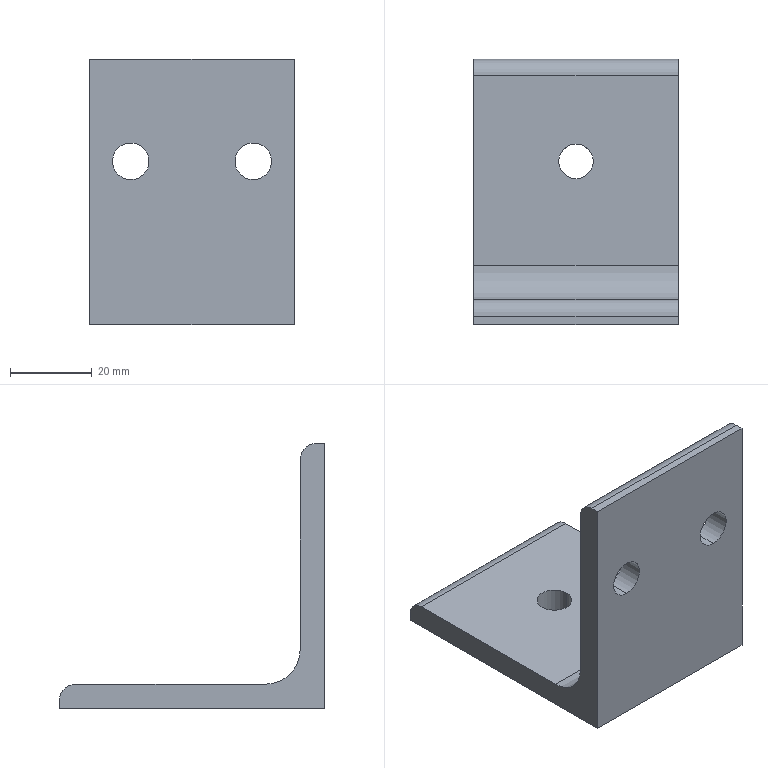Part | STEP file | 0245_204_Blacket | 1 solid | 17 faces | box 50 x 65 x 65 mm | volume 36528 mm3 | cylinder 9 | plane 8 | commonest cylinder face diameters 9 x4 8 x2 8.5 x2 17 x1
STEP:
#1=CARTESIAN_POINT('',(0.,0.,0.));
#2=DIRECTION('',(0.,0.,1.));
#3=DIRECTION('',(1.,0.,0.));
#4=AXIS2_PLACEMENT_3D('',#1,#2,#3);
#5=CARTESIAN_POINT('',(4.25,40.,-65.));
#6=VERTEX_POINT('',#5);
#7=CARTESIAN_POINT('',(4.25,40.,-59.));
#8=VERTEX_POINT('',#7);
#9=CARTESIAN_POINT('',(4.25,40.,-59.));
#10=DIRECTION('',(0.,0.,1.));
#11=VECTOR('',#10,1.);
#12=LINE('',#9,#11);
#13=CARTESIAN_POINT('',(0.,40.,-59.));
#14=DIRECTION('',(0.,0.,1.));
#15=DIRECTION('',(1.,0.,0.));
#16=AXIS2_PLACEMENT_3D('',#13,#14,#15);
#17=CYLINDRICAL_SURFACE('',#16,4.25);
#18=CARTESIAN_POINT('',(6.283,0.));
#19=DIRECTION('',(0.,1.));
#20=VECTOR('',#19,1.);
#21=LINE('',#18,#20);
#22=(GEOMETRIC_REPRESENTATION_CONTEXT(2)PARAMETRIC_REPRESENTATION_CONTEXT()REPRESENTATION_CONTEXT('',''));
#23=DEFINITIONAL_REPRESENTATION('',(#21),#22);
#24=PCURVE('',#17,#23);
#25=CARTESIAN_POINT('',(0.,40.,-59.));
#26=DIRECTION('',(0.,0.,1.));
#27=DIRECTION('',(1.,0.,0.));
#28=AXIS2_PLACEMENT_3D('',#25,#26,#27);
#29=CYLINDRICAL_SURFACE('',#28,4.25);
#30=CARTESIAN_POINT('',(0.,0.));
#31=DIRECTION('',(0.,1.));
#32=VECTOR('',#31,1.);
#33=LINE('',#30,#32);
#34=(GEOMETRIC_REPRESENTATION_CONTEXT(2)PARAMETRIC_REPRESENTATION_CONTEXT()REPRESENTATION_CONTEXT('',''));
#35=DEFINITIONAL_REPRESENTATION('',(#33),#34);
#36=PCURVE('',#29,#35);
#37=SURFACE_CURVE('',#12,(#24,#36),.PCURVE_S1.);
#38=EDGE_CURVE('',#6,#8,#37,.T.);
#39=ORIENTED_EDGE('',*,*,#38,.T.);
#40=CARTESIAN_POINT('',(-4.25,40.,-59.));
#41=VERTEX_POINT('',#40);
#42=CARTESIAN_POINT('',(0.,40.,-59.));
#43=DIRECTION('',(0.,0.,1.));
#44=DIRECTION('',(1.,0.,0.));
#45=AXIS2_PLACEMENT_3D('',#42,#43,#44);
#46=CIRCLE('',#45,4.25);
#47=CARTESIAN_POINT('',(0.,0.));
#48=DIRECTION('',(1.,0.));
#49=VECTOR('',#48,1.);
#50=LINE('',#47,#49);
#51=(GEOMETRIC_REPRESENTATION_CONTEXT(2)PARAMETRIC_REPRESENTATION_CONTEXT()REPRESENTATION_CONTEXT('',''));
#52=DEFINITIONAL_REPRESENTATION('',(#50),#51);
#53=PCURVE('',#17,#52);
#54=CARTESIAN_POINT('',(25.,65.,-59.));
#55=DIRECTION('',(0.,0.,-1.));
#56=DIRECTION('',(0.,1.,0.));
#57=AXIS2_PLACEMENT_3D('',#54,#55,#56);
#58=PLANE('',#57);
#59=CARTESIAN_POINT('',(-25.,-20.75));
#60=CARTESIAN_POINT('',(-17.639,-20.75));
#61=CARTESIAN_POINT('',(-21.319,-27.125));
#62=CARTESIAN_POINT('',(-25.,-33.5));
#63=CARTESIAN_POINT('',(-28.681,-27.125));
#64=CARTESIAN_POINT('',(-32.361,-20.75));
#65=CARTESIAN_POINT('',(-25.,-20.75));
#66=(BOUNDED_CURVE()B_SPLINE_CURVE(2,(#59,#60,#61,#62,#63,#64,#65),.UNSPECIFIED.,.T.,.F.)B_SPLINE_CURVE_WITH_KNOTS((1,2,2,2,2,1),(-2.094,0.,2.094,4.189,6.283,8.378),.UNSPECIFIED.)CURVE()GEOMETRIC_REPRESENTATION_ITEM()RATIONAL_B_SPLINE_CURVE((1.,0.5,1.,0.5,1.,0.5,1.))REPRESENTATION_ITEM(''));
#67=(GEOMETRIC_REPRESENTATION_CONTEXT(2)PARAMETRIC_REPRESENTATION_CONTEXT()REPRESENTATION_CONTEXT('',''));
#68=DEFINITIONAL_REPRESENTATION('',(#66),#67);
#69=PCURVE('',#58,#68);
#70=SURFACE_CURVE('',#46,(#53,#69),.PCURVE_S1.);
#71=EDGE_CURVE('',#41,#8,#70,.T.);
#72=ORIENTED_EDGE('',*,*,#71,.F.);
#73=CARTESIAN_POINT('',(-4.25,40.,-65.));
#74=VERTEX_POINT('',#73);
#75=CARTESIAN_POINT('',(-4.25,40.,-59.));
#76=DIRECTION('',(0.,0.,1.));
#77=VECTOR('',#76,1.);
#78=LINE('',#75,#77);
#79=CARTESIAN_POINT('',(3.142,0.));
#80=DIRECTION('',(0.,1.));
#81=VECTOR('',#80,1.);
#82=LINE('',#79,#81);
#83=(GEOMETRIC_REPRESENTATION_CONTEXT(2)PARAMETRIC_REPRESENTATION_CONTEXT()REPRESENTATION_CONTEXT('',''));
#84=DEFINITIONAL_REPRESENTATION('',(#82),#83);
#85=PCURVE('',#17,#84);
#86=CARTESIAN_POINT('',(3.142,0.));
#87=DIRECTION('',(0.,1.));
#88=VECTOR('',#87,1.);
#89=LINE('',#86,#88);
#90=(GEOMETRIC_REPRESENTATION_CONTEXT(2)PARAMETRIC_REPRESENTATION_CONTEXT()REPRESENTATION_CONTEXT('',''));
#91=DEFINITIONAL_REPRESENTATION('',(#89),#90);
#92=PCURVE('',#29,#91);
#93=SURFACE_CURVE('',#78,(#85,#92),.PCURVE_S1.);
#94=EDGE_CURVE('',#74,#41,#93,.T.);
#95=ORIENTED_EDGE('',*,*,#94,.F.);
#96=CARTESIAN_POINT('',(0.,40.,-65.));
#97=DIRECTION('',(0.,0.,1.));
#98=DIRECTION('',(1.,0.,0.));
#99=AXIS2_PLACEMENT_3D('',#96,#97,#98);
#100=CIRCLE('',#99,4.25);
#101=CARTESIAN_POINT('',(0.,-6.));
#102=DIRECTION('',(1.,0.));
#103=VECTOR('',#102,1.);
#104=LINE('',#101,#103);
#105=(GEOMETRIC_REPRESENTATION_CONTEXT(2)PARAMETRIC_REPRESENTATION_CONTEXT()REPRESENTATION_CONTEXT('',''));
#106=DEFINITIONAL_REPRESENTATION('',(#104),#105);
#107=PCURVE('',#17,#106);
#108=CARTESIAN_POINT('',(25.,0.,-65.));
#109=DIRECTION('',(0.,0.,1.));
#110=DIRECTION('',(1.,0.,0.));
#111=AXIS2_PLACEMENT_3D('',#108,#109,#110);
#112=PLANE('',#111);
#113=CARTESIAN_POINT('',(-25.,40.));
#114=DIRECTION('',(1.,0.));
#115=AXIS2_PLACEMENT_2D('',#113,#114);
#116=CIRCLE('',#115,4.25);
#117=(GEOMETRIC_REPRESENTATION_CONTEXT(2)PARAMETRIC_REPRESENTATION_CONTEXT()REPRESENTATION_CONTEXT('',''));
#118=DEFINITIONAL_REPRESENTATION('',(#116),#117);
#119=PCURVE('',#112,#118);
#120=SURFACE_CURVE('',#100,(#107,#119),.PCURVE_S1.);
#121=EDGE_CURVE('',#74,#6,#120,.T.);
#122=ORIENTED_EDGE('',*,*,#121,.T.);
#123=EDGE_LOOP('',(#39,#72,#95,#122));
#124=FACE_BOUND('',#123,.F.);
#125=ADVANCED_FACE('',(#124),#17,.F.);
#126=CARTESIAN_POINT('',(-15.,0.,-20.5));
#127=VERTEX_POINT('',#126);
#128=CARTESIAN_POINT('',(-15.,6.,-20.5));
#129=VERTEX_POINT('',#128);
#130=CARTESIAN_POINT('',(-15.,6.,-20.5));
#131=DIRECTION('',(0.,1.,0.));
#132=VECTOR('',#131,1.);
#133=LINE('',#130,#132);
#134=CARTESIAN_POINT('',(-15.,6.,-25.));
#135=DIRECTION('',(0.,1.,0.));
#136=DIRECTION('',(0.,0.,1.));
#137=AXIS2_PLACEMENT_3D('',#134,#135,#136);
#138=CYLINDRICAL_SURFACE('',#137,4.5);
#139=CARTESIAN_POINT('',(6.283,0.));
#140=DIRECTION('',(0.,1.));
#141=VECTOR('',#140,1.);
#142=LINE('',#139,#141);
#143=(GEOMETRIC_REPRESENTATION_CONTEXT(2)PARAMETRIC_REPRESENTATION_CONTEXT()REPRESENTATION_CONTEXT('',''));
#144=DEFINITIONAL_REPRESENTATION('',(#142),#143);
#145=PCURVE('',#138,#144);
#146=CARTESIAN_POINT('',(-15.,6.,-25.));
#147=DIRECTION('',(0.,1.,0.));
#148=DIRECTION('',(0.,0.,1.));
#149=AXIS2_PLACEMENT_3D('',#146,#147,#148);
#150=CYLINDRICAL_SURFACE('',#149,4.5);
#151=CARTESIAN_POINT('',(0.,0.));
#152=DIRECTION('',(0.,1.));
#153=VECTOR('',#152,1.);
#154=LINE('',#151,#153);
#155=(GEOMETRIC_REPRESENTATION_CONTEXT(2)PARAMETRIC_REPRESENTATION_CONTEXT()REPRESENTATION_CONTEXT('',''));
#156=DEFINITIONAL_REPRESENTATION('',(#154),#155);
#157=PCURVE('',#150,#156);
#158=SURFACE_CURVE('',#133,(#145,#157),.PCURVE_S1.);
#159=EDGE_CURVE('',#127,#129,#158,.T.);
#160=ORIENTED_EDGE('',*,*,#159,.T.);
#161=CARTESIAN_POINT('',(-15.,6.,-29.5));
#162=VERTEX_POINT('',#161);
#163=CARTESIAN_POINT('',(-15.,6.,-25.));
#164=DIRECTION('',(0.,1.,0.));
#165=DIRECTION('',(0.,0.,1.));
#166=AXIS2_PLACEMENT_3D('',#163,#164,#165);
#167=CIRCLE('',#166,4.5);
#168=CARTESIAN_POINT('',(0.,0.));
#169=DIRECTION('',(1.,0.));
#170=VECTOR('',#169,1.);
#171=LINE('',#168,#170);
#172=(GEOMETRIC_REPRESENTATION_CONTEXT(2)PARAMETRIC_REPRESENTATION_CONTEXT()REPRESENTATION_CONTEXT('',''));
#173=DEFINITIONAL_REPRESENTATION('',(#171),#172);
#174=PCURVE('',#138,#173);
#175=CARTESIAN_POINT('',(25.,6.,-59.));
#176=DIRECTION('',(0.,-1.,0.));
#177=DIRECTION('',(0.,0.,-1.));
#178=AXIS2_PLACEMENT_3D('',#175,#176,#177);
#179=PLANE('',#178);
#180=CARTESIAN_POINT('',(-38.5,-40.));
#181=CARTESIAN_POINT('',(-38.5,-32.206));
#182=CARTESIAN_POINT('',(-31.75,-36.103));
#183=CARTESIAN_POINT('',(-25.,-40.));
#184=CARTESIAN_POINT('',(-31.75,-43.897));
#185=CARTESIAN_POINT('',(-38.5,-47.794));
#186=CARTESIAN_POINT('',(-38.5,-40.));
#187=(BOUNDED_CURVE()B_SPLINE_CURVE(2,(#180,#181,#182,#183,#184,#185,#186),.UNSPECIFIED.,.T.,.F.)B_SPLINE_CURVE_WITH_KNOTS((1,2,2,2,2,1),(-2.094,0.,2.094,4.189,6.283,8.378),.UNSPECIFIED.)CURVE()GEOMETRIC_REPRESENTATION_ITEM()RATIONAL_B_SPLINE_CURVE((1.,0.5,1.,0.5,1.,0.5,1.))REPRESENTATION_ITEM(''));
#188=(GEOMETRIC_REPRESENTATION_CONTEXT(2)PARAMETRIC_REPRESENTATION_CONTEXT()REPRESENTATION_CONTEXT('',''));
#189=DEFINITIONAL_REPRESENTATION('',(#187),#188);
#190=PCURVE('',#179,#189);
#191=SURFACE_CURVE('',#167,(#174,#190),.PCURVE_S1.);
#192=EDGE_CURVE('',#162,#129,#191,.T.);
#193=ORIENTED_EDGE('',*,*,#192,.F.);
#194=CARTESIAN_POINT('',(-15.,0.,-29.5));
#195=VERTEX_POINT('',#194);
#196=CARTESIAN_POINT('',(-15.,6.,-29.5));
#197=DIRECTION('',(0.,1.,0.));
#198=VECTOR('',#197,1.);
#199=LINE('',#196,#198);
#200=CARTESIAN_POINT('',(3.142,0.));
#201=DIRECTION('',(0.,1.));
#202=VECTOR('',#201,1.);
#203=LINE('',#200,#202);
#204=(GEOMETRIC_REPRESENTATION_CONTEXT(2)PARAMETRIC_REPRESENTATION_CONTEXT()REPRESENTATION_CONTEXT('',''));
#205=DEFINITIONAL_REPRESENTATION('',(#203),#204);
#206=PCURVE('',#138,#205);
#207=CARTESIAN_POINT('',(3.142,0.));
#208=DIRECTION('',(0.,1.));
#209=VECTOR('',#208,1.);
#210=LINE('',#207,#209);
#211=(GEOMETRIC_REPRESENTATION_CONTEXT(2)PARAMETRIC_REPRESENTATION_CONTEXT()REPRESENTATION_CONTEXT('',''));
#212=DEFINITIONAL_REPRESENTATION('',(#210),#211);
#213=PCURVE('',#150,#212);
#214=SURFACE_CURVE('',#199,(#206,#213),.PCURVE_S1.);
#215=EDGE_CURVE('',#195,#162,#214,.T.);
#216=ORIENTED_EDGE('',*,*,#215,.F.);
#217=CARTESIAN_POINT('',(-15.,0.,-25.));
#218=DIRECTION('',(0.,1.,0.));
#219=DIRECTION('',(0.,0.,1.));
#220=AXIS2_PLACEMENT_3D('',#217,#218,#219);
#221=CIRCLE('',#220,4.5);
#222=CARTESIAN_POINT('',(0.,-6.));
#223=DIRECTION('',(1.,0.));
#224=VECTOR('',#223,1.);
#225=LINE('',#222,#224);
#226=(GEOMETRIC_REPRESENTATION_CONTEXT(2)PARAMETRIC_REPRESENTATION_CONTEXT()REPRESENTATION_CONTEXT('',''));
#227=DEFINITIONAL_REPRESENTATION('',(#225),#226);
#228=PCURVE('',#138,#227);
#229=CARTESIAN_POINT('',(25.,0.,0.));
#230=DIRECTION('',(0.,1.,0.));
#231=DIRECTION('',(0.,0.,1.));
#232=AXIS2_PLACEMENT_3D('',#229,#230,#231);
#233=PLANE('',#232);
#234=CARTESIAN_POINT('',(-25.,-40.));
#235=DIRECTION('',(1.,0.));
#236=AXIS2_PLACEMENT_2D('',#234,#235);
#237=CIRCLE('',#236,4.5);
#238=(GEOMETRIC_REPRESENTATION_CONTEXT(2)PARAMETRIC_REPRESENTATION_CONTEXT()REPRESENTATION_CONTEXT('',''));
#239=DEFINITIONAL_REPRESENTATION('',(#237),#238);
#240=PCURVE('',#233,#239);
#241=SURFACE_CURVE('',#221,(#228,#240),.PCURVE_S1.);
#242=EDGE_CURVE('',#195,#127,#241,.T.);
#243=ORIENTED_EDGE('',*,*,#242,.T.);
#244=EDGE_LOOP('',(#160,#193,#216,#243));
#245=FACE_BOUND('',#244,.F.);
#246=ADVANCED_FACE('',(#245),#138,.F.);
#247=CARTESIAN_POINT('',(15.,0.,-20.5));
#248=VERTEX_POINT('',#247);
#249=CARTESIAN_POINT('',(15.,6.,-20.5));
#250=VERTEX_POINT('',#249);
#251=CARTESIAN_POINT('',(15.,6.,-20.5));
#252=DIRECTION('',(0.,1.,0.));
#253=VECTOR('',#252,1.);
#254=LINE('',#251,#253);
#255=CARTESIAN_POINT('',(15.,6.,-25.));
#256=DIRECTION('',(0.,1.,0.));
#257=DIRECTION('',(0.,0.,1.));
#258=AXIS2_PLACEMENT_3D('',#255,#256,#257);
#259=CYLINDRICAL_SURFACE('',#258,4.5);
#260=CARTESIAN_POINT('',(6.283,0.));
#261=DIRECTION('',(0.,1.));
#262=VECTOR('',#261,1.);
#263=LINE('',#260,#262);
#264=(GEOMETRIC_REPRESENTATION_CONTEXT(2)PARAMETRIC_REPRESENTATION_CONTEXT()REPRESENTATION_CONTEXT('',''));
#265=DEFINITIONAL_REPRESENTATION('',(#263),#264);
#266=PCURVE('',#259,#265);
#267=CARTESIAN_POINT('',(15.,6.,-25.));
#268=DIRECTION('',(0.,1.,0.));
#269=DIRECTION('',(0.,0.,1.));
#270=AXIS2_PLACEMENT_3D('',#267,#268,#269);
#271=CYLINDRICAL_SURFACE('',#270,4.5);
#272=CARTESIAN_POINT('',(0.,0.));
#273=DIRECTION('',(0.,1.));
#274=VECTOR('',#273,1.);
#275=LINE('',#272,#274);
#276=(GEOMETRIC_REPRESENTATION_CONTEXT(2)PARAMETRIC_REPRESENTATION_CONTEXT()REPRESENTATION_CONTEXT('',''));
#277=DEFINITIONAL_REPRESENTATION('',(#275),#276);
#278=PCURVE('',#271,#277);
#279=SURFACE_CURVE('',#254,(#266,#278),.PCURVE_S1.);
#280=EDGE_CURVE('',#248,#250,#279,.T.);
#281=ORIENTED_EDGE('',*,*,#280,.T.);
#282=CARTESIAN_POINT('',(15.,6.,-29.5));
#283=VERTEX_POINT('',#282);
#284=CARTESIAN_POINT('',(15.,6.,-25.));
#285=DIRECTION('',(0.,1.,0.));
#286=DIRECTION('',(0.,0.,1.));
#287=AXIS2_PLACEMENT_3D('',#284,#285,#286);
#288=CIRCLE('',#287,4.5);
#289=CARTESIAN_POINT('',(0.,0.));
#290=DIRECTION('',(1.,0.));
#291=VECTOR('',#290,1.);
#292=LINE('',#289,#291);
#293=(GEOMETRIC_REPRESENTATION_CONTEXT(2)PARAMETRIC_REPRESENTATION_CONTEXT()REPRESENTATION_CONTEXT('',''));
#294=DEFINITIONAL_REPRESENTATION('',(#292),#293);
#295=PCURVE('',#259,#294);
#296=CARTESIAN_POINT('',(-38.5,-10.));
#297=CARTESIAN_POINT('',(-38.5,-2.206));
#298=CARTESIAN_POINT('',(-31.75,-6.103));
#299=CARTESIAN_POINT('',(-25.,-10.));
#300=CARTESIAN_POINT('',(-31.75,-13.897));
#301=CARTESIAN_POINT('',(-38.5,-17.794));
#302=CARTESIAN_POINT('',(-38.5,-10.));
#303=(BOUNDED_CURVE()B_SPLINE_CURVE(2,(#296,#297,#298,#299,#300,#301,#302),.UNSPECIFIED.,.T.,.F.)B_SPLINE_CURVE_WITH_KNOTS((1,2,2,2,2,1),(-2.094,0.,2.094,4.189,6.283,8.378),.UNSPECIFIED.)CURVE()GEOMETRIC_REPRESENTATION_ITEM()RATIONAL_B_SPLINE_CURVE((1.,0.5,1.,0.5,1.,0.5,1.))REPRESENTATION_ITEM(''));
#304=(GEOMETRIC_REPRESENTATION_CONTEXT(2)PARAMETRIC_REPRESENTATION_CONTEXT()REPRESENTATION_CONTEXT('',''));
#305=DEFINITIONAL_REPRESENTATION('',(#303),#304);
#306=PCURVE('',#179,#305);
#307=SURFACE_CURVE('',#288,(#295,#306),.PCURVE_S1.);
#308=EDGE_CURVE('',#283,#250,#307,.T.);
#309=ORIENTED_EDGE('',*,*,#308,.F.);
#310=CARTESIAN_POINT('',(15.,0.,-29.5));
#311=VERTEX_POINT('',#310);
#312=CARTESIAN_POINT('',(15.,6.,-29.5));
#313=DIRECTION('',(0.,1.,0.));
#314=VECTOR('',#313,1.);
#315=LINE('',#312,#314);
#316=CARTESIAN_POINT('',(3.142,0.));
#317=DIRECTION('',(0.,1.));
#318=VECTOR('',#317,1.);
#319=LINE('',#316,#318);
#320=(GEOMETRIC_REPRESENTATION_CONTEXT(2)PARAMETRIC_REPRESENTATION_CONTEXT()REPRESENTATION_CONTEXT('',''));
#321=DEFINITIONAL_REPRESENTATION('',(#319),#320);
#322=PCURVE('',#259,#321);
#323=CARTESIAN_POINT('',(3.142,0.));
#324=DIRECTION('',(0.,1.));
#325=VECTOR('',#324,1.);
#326=LINE('',#323,#325);
#327=(GEOMETRIC_REPRESENTATION_CONTEXT(2)PARAMETRIC_REPRESENTATION_CONTEXT()REPRESENTATION_CONTEXT('',''));
#328=DEFINITIONAL_REPRESENTATION('',(#326),#327);
#329=PCURVE('',#271,#328);
#330=SURFACE_CURVE('',#315,(#322,#329),.PCURVE_S1.);
#331=EDGE_CURVE('',#311,#283,#330,.T.);
#332=ORIENTED_EDGE('',*,*,#331,.F.);
#333=CARTESIAN_POINT('',(15.,0.,-25.));
#334=DIRECTION('',(0.,1.,0.));
#335=DIRECTION('',(0.,0.,1.));
#336=AXIS2_PLACEMENT_3D('',#333,#334,#335);
#337=CIRCLE('',#336,4.5);
#338=CARTESIAN_POINT('',(0.,-6.));
#339=DIRECTION('',(1.,0.));
#340=VECTOR('',#339,1.);
#341=LINE('',#338,#340);
#342=(GEOMETRIC_REPRESENTATION_CONTEXT(2)PARAMETRIC_REPRESENTATION_CONTEXT()REPRESENTATION_CONTEXT('',''));
#343=DEFINITIONAL_REPRESENTATION('',(#341),#342);
#344=PCURVE('',#259,#343);
#345=CARTESIAN_POINT('',(-25.,-10.));
#346=DIRECTION('',(1.,0.));
#347=AXIS2_PLACEMENT_2D('',#345,#346);
#348=CIRCLE('',#347,4.5);
#349=(GEOMETRIC_REPRESENTATION_CONTEXT(2)PARAMETRIC_REPRESENTATION_CONTEXT()REPRESENTATION_CONTEXT('',''));
#350=DEFINITIONAL_REPRESENTATION('',(#348),#349);
#351=PCURVE('',#233,#350);
#352=SURFACE_CURVE('',#337,(#344,#351),.PCURVE_S1.);
#353=EDGE_CURVE('',#311,#248,#352,.T.);
#354=ORIENTED_EDGE('',*,*,#353,.T.);
#355=EDGE_LOOP('',(#281,#309,#332,#354));
#356=FACE_BOUND('',#355,.F.);
#357=ADVANCED_FACE('',(#356),#259,.F.);
#358=CARTESIAN_POINT('',(25.,2.,0.));
#359=VERTEX_POINT('',#358);
#360=CARTESIAN_POINT('',(25.,0.,0.));
#361=VERTEX_POINT('',#360);
#362=CARTESIAN_POINT('',(25.,6.,0.));
#363=DIRECTION('',(0.,-1.,0.));
#364=VECTOR('',#363,1.);
#365=LINE('',#362,#364);
#366=CARTESIAN_POINT('',(25.,6.,0.));
#367=DIRECTION('',(0.,0.,-1.));
#368=DIRECTION('',(0.,1.,0.));
#369=AXIS2_PLACEMENT_3D('',#366,#367,#368);
#370=PLANE('',#369);
#371=CARTESIAN_POINT('',(0.,0.));
#372=DIRECTION('',(-1.,0.));
#373=VECTOR('',#372,1.);
#374=LINE('',#371,#373);
#375=(GEOMETRIC_REPRESENTATION_CONTEXT(2)PARAMETRIC_REPRESENTATION_CONTEXT()REPRESENTATION_CONTEXT('',''));
#376=DEFINITIONAL_REPRESENTATION('',(#374),#375);
#377=PCURVE('',#370,#376);
#378=CARTESIAN_POINT('',(25.,0.,0.));
#379=DIRECTION('',(1.,0.,0.));
#380=DIRECTION('',(0.,0.,-1.));
#381=AXIS2_PLACEMENT_3D('',#378,#379,#380);
#382=PLANE('',#381);
#383=CARTESIAN_POINT('',(0.,6.));
#384=DIRECTION('',(0.,-1.));
#385=VECTOR('',#384,1.);
#386=LINE('',#383,#385);
#387=(GEOMETRIC_REPRESENTATION_CONTEXT(2)PARAMETRIC_REPRESENTATION_CONTEXT()REPRESENTATION_CONTEXT('',''));
#388=DEFINITIONAL_REPRESENTATION('',(#386),#387);
#389=PCURVE('',#382,#388);
#390=SURFACE_CURVE('',#365,(#377,#389),.PCURVE_S1.);
#391=EDGE_CURVE('',#359,#361,#390,.T.);
#392=ORIENTED_EDGE('',*,*,#391,.F.);
#393=CARTESIAN_POINT('',(-25.,2.,0.));
#394=VERTEX_POINT('',#393);
#395=CARTESIAN_POINT('',(25.,2.,0.));
#396=DIRECTION('',(-1.,0.,0.));
#397=VECTOR('',#396,1.);
#398=LINE('',#395,#397);
#399=CARTESIAN_POINT('',(-4.,0.));
#400=DIRECTION('',(0.,-1.));
#401=VECTOR('',#400,1.);
#402=LINE('',#399,#401);
#403=(GEOMETRIC_REPRESENTATION_CONTEXT(2)PARAMETRIC_REPRESENTATION_CONTEXT()REPRESENTATION_CONTEXT('',''));
#404=DEFINITIONAL_REPRESENTATION('',(#402),#403);
#405=PCURVE('',#370,#404);
#406=CARTESIAN_POINT('',(25.,2.,-4.));
#407=DIRECTION('',(-1.,0.,0.));
#408=DIRECTION('',(0.,0.,1.));
#409=AXIS2_PLACEMENT_3D('',#406,#407,#408);
#410=CYLINDRICAL_SURFACE('',#409,4.);
#411=CARTESIAN_POINT('',(0.,0.));
#412=DIRECTION('',(0.,1.));
#413=VECTOR('',#412,1.);
#414=LINE('',#411,#413);
#415=(GEOMETRIC_REPRESENTATION_CONTEXT(2)PARAMETRIC_REPRESENTATION_CONTEXT()REPRESENTATION_CONTEXT('',''));
#416=DEFINITIONAL_REPRESENTATION('',(#414),#415);
#417=PCURVE('',#410,#416);
#418=SURFACE_CURVE('',#398,(#405,#417),.PCURVE_S1.);
#419=EDGE_CURVE('',#359,#394,#418,.T.);
#420=ORIENTED_EDGE('',*,*,#419,.T.);
#421=CARTESIAN_POINT('',(-25.,0.,0.));
#422=VERTEX_POINT('',#421);
#423=CARTESIAN_POINT('',(-25.,6.,0.));
#424=DIRECTION('',(0.,-1.,0.));
#425=VECTOR('',#424,1.);
#426=LINE('',#423,#425);
#427=CARTESIAN_POINT('',(0.,-50.));
#428=DIRECTION('',(-1.,0.));
#429=VECTOR('',#428,1.);
#430=LINE('',#427,#429);
#431=(GEOMETRIC_REPRESENTATION_CONTEXT(2)PARAMETRIC_REPRESENTATION_CONTEXT()REPRESENTATION_CONTEXT('',''));
#432=DEFINITIONAL_REPRESENTATION('',(#430),#431);
#433=PCURVE('',#370,#432);
#434=CARTESIAN_POINT('',(-25.,0.,0.));
#435=DIRECTION('',(1.,0.,0.));
#436=DIRECTION('',(0.,0.,-1.));
#437=AXIS2_PLACEMENT_3D('',#434,#435,#436);
#438=PLANE('',#437);
#439=CARTESIAN_POINT('',(0.,6.));
#440=DIRECTION('',(0.,-1.));
#441=VECTOR('',#440,1.);
#442=LINE('',#439,#441);
#443=(GEOMETRIC_REPRESENTATION_CONTEXT(2)PARAMETRIC_REPRESENTATION_CONTEXT()REPRESENTATION_CONTEXT('',''));
#444=DEFINITIONAL_REPRESENTATION('',(#442),#443);
#445=PCURVE('',#438,#444);
#446=SURFACE_CURVE('',#426,(#433,#445),.PCURVE_S1.);
#447=EDGE_CURVE('',#394,#422,#446,.T.);
#448=ORIENTED_EDGE('',*,*,#447,.T.);
#449=CARTESIAN_POINT('',(25.,0.,0.));
#450=DIRECTION('',(-1.,0.,0.));
#451=VECTOR('',#450,1.);
#452=LINE('',#449,#451);
#453=CARTESIAN_POINT('',(-6.,0.));
#454=DIRECTION('',(0.,-1.));
#455=VECTOR('',#454,1.);
#456=LINE('',#453,#455);
#457=(GEOMETRIC_REPRESENTATION_CONTEXT(2)PARAMETRIC_REPRESENTATION_CONTEXT()REPRESENTATION_CONTEXT('',''));
#458=DEFINITIONAL_REPRESENTATION('',(#456),#457);
#459=PCURVE('',#370,#458);
#460=CARTESIAN_POINT('',(0.,0.));
#461=DIRECTION('',(0.,-1.));
#462=VECTOR('',#461,1.);
#463=LINE('',#460,#462);
#464=(GEOMETRIC_REPRESENTATION_CONTEXT(2)PARAMETRIC_REPRESENTATION_CONTEXT()REPRESENTATION_CONTEXT('',''));
#465=DEFINITIONAL_REPRESENTATION('',(#463),#464);
#466=PCURVE('',#233,#465);
#467=SURFACE_CURVE('',#452,(#459,#466),.PCURVE_S1.);
#468=EDGE_CURVE('',#361,#422,#467,.T.);
#469=ORIENTED_EDGE('',*,*,#468,.F.);
#470=EDGE_LOOP('',(#392,#420,#448,#469));
#471=FACE_BOUND('',#470,.T.);
#472=ADVANCED_FACE('',(#471),#370,.F.);
#473=CARTESIAN_POINT('',(-15.,0.,-25.));
#474=DIRECTION('',(0.,1.,0.));
#475=DIRECTION('',(0.,0.,1.));
#476=AXIS2_PLACEMENT_3D('',#473,#474,#475);
#477=CIRCLE('',#476,4.5);
#478=CARTESIAN_POINT('',(-25.,-40.));
#479=DIRECTION('',(1.,0.));
#480=AXIS2_PLACEMENT_2D('',#478,#479);
#481=CIRCLE('',#480,4.5);
#482=(GEOMETRIC_REPRESENTATION_CONTEXT(2)PARAMETRIC_REPRESENTATION_CONTEXT()REPRESENTATION_CONTEXT('',''));
#483=DEFINITIONAL_REPRESENTATION('',(#481),#482);
#484=PCURVE('',#233,#483);
#485=CARTESIAN_POINT('',(0.,-6.));
#486=DIRECTION('',(1.,0.));
#487=VECTOR('',#486,1.);
#488=LINE('',#485,#487);
#489=(GEOMETRIC_REPRESENTATION_CONTEXT(2)PARAMETRIC_REPRESENTATION_CONTEXT()REPRESENTATION_CONTEXT('',''));
#490=DEFINITIONAL_REPRESENTATION('',(#488),#489);
#491=PCURVE('',#150,#490);
#492=SURFACE_CURVE('',#477,(#484,#491),.PCURVE_S1.);
#493=EDGE_CURVE('',#127,#195,#492,.T.);
#494=ORIENTED_EDGE('',*,*,#493,.T.);
#495=ORIENTED_EDGE('',*,*,#242,.T.);
#496=EDGE_LOOP('',(#494,#495));
#497=FACE_BOUND('',#496,.T.);
#498=CARTESIAN_POINT('',(15.,0.,-25.));
#499=DIRECTION('',(0.,1.,0.));
#500=DIRECTION('',(0.,0.,1.));
#501=AXIS2_PLACEMENT_3D('',#498,#499,#500);
#502=CIRCLE('',#501,4.5);
#503=CARTESIAN_POINT('',(-25.,-10.));
#504=DIRECTION('',(1.,0.));
#505=AXIS2_PLACEMENT_2D('',#503,#504);
#506=CIRCLE('',#505,4.5);
#507=(GEOMETRIC_REPRESENTATION_CONTEXT(2)PARAMETRIC_REPRESENTATION_CONTEXT()REPRESENTATION_CONTEXT('',''));
#508=DEFINITIONAL_REPRESENTATION('',(#506),#507);
#509=PCURVE('',#233,#508);
#510=CARTESIAN_POINT('',(0.,-6.));
#511=DIRECTION('',(1.,0.));
#512=VECTOR('',#511,1.);
#513=LINE('',#510,#512);
#514=(GEOMETRIC_REPRESENTATION_CONTEXT(2)PARAMETRIC_REPRESENTATION_CONTEXT()REPRESENTATION_CONTEXT('',''));
#515=DEFINITIONAL_REPRESENTATION('',(#513),#514);
#516=PCURVE('',#271,#515);
#517=SURFACE_CURVE('',#502,(#509,#516),.PCURVE_S1.);
#518=EDGE_CURVE('',#248,#311,#517,.T.);
#519=ORIENTED_EDGE('',*,*,#518,.T.);
#520=ORIENTED_EDGE('',*,*,#353,.T.);
#521=EDGE_LOOP('',(#519,#520));
#522=FACE_BOUND('',#521,.T.);
#523=CARTESIAN_POINT('',(-25.,0.,-65.));
#524=VERTEX_POINT('',#523);
#525=CARTESIAN_POINT('',(-25.,0.,0.));
#526=DIRECTION('',(0.,0.,-1.));
#527=VECTOR('',#526,1.);
#528=LINE('',#525,#527);
#529=CARTESIAN_POINT('',(0.,-50.));
#530=DIRECTION('',(-1.,0.));
#531=VECTOR('',#530,1.);
#532=LINE('',#529,#531);
#533=(GEOMETRIC_REPRESENTATION_CONTEXT(2)PARAMETRIC_REPRESENTATION_CONTEXT()REPRESENTATION_CONTEXT('',''));
#534=DEFINITIONAL_REPRESENTATION('',(#532),#533);
#535=PCURVE('',#233,#534);
#536=CARTESIAN_POINT('',(0.,0.));
#537=DIRECTION('',(1.,0.));
#538=VECTOR('',#537,1.);
#539=LINE('',#536,#538);
#540=(GEOMETRIC_REPRESENTATION_CONTEXT(2)PARAMETRIC_REPRESENTATION_CONTEXT()REPRESENTATION_CONTEXT('',''));
#541=DEFINITIONAL_REPRESENTATION('',(#539),#540);
#542=PCURVE('',#438,#541);
#543=SURFACE_CURVE('',#528,(#535,#542),.PCURVE_S1.);
#544=EDGE_CURVE('',#422,#524,#543,.T.);
#545=ORIENTED_EDGE('',*,*,#544,.T.);
#546=CARTESIAN_POINT('',(25.,0.,-65.));
#547=VERTEX_POINT('',#546);
#548=CARTESIAN_POINT('',(25.,0.,-65.));
#549=DIRECTION('',(-1.,0.,0.));
#550=VECTOR('',#549,1.);
#551=LINE('',#548,#550);
#552=CARTESIAN_POINT('',(-65.,0.));
#553=DIRECTION('',(0.,-1.));
#554=VECTOR('',#553,1.);
#555=LINE('',#552,#554);
#556=(GEOMETRIC_REPRESENTATION_CONTEXT(2)PARAMETRIC_REPRESENTATION_CONTEXT()REPRESENTATION_CONTEXT('',''));
#557=DEFINITIONAL_REPRESENTATION('',(#555),#556);
#558=PCURVE('',#233,#557);
#559=CARTESIAN_POINT('',(0.,0.));
#560=DIRECTION('',(-1.,0.));
#561=VECTOR('',#560,1.);
#562=LINE('',#559,#561);
#563=(GEOMETRIC_REPRESENTATION_CONTEXT(2)PARAMETRIC_REPRESENTATION_CONTEXT()REPRESENTATION_CONTEXT('',''));
#564=DEFINITIONAL_REPRESENTATION('',(#562),#563);
#565=PCURVE('',#112,#564);
#566=SURFACE_CURVE('',#551,(#558,#565),.PCURVE_S1.);
#567=EDGE_CURVE('',#547,#524,#566,.T.);
#568=ORIENTED_EDGE('',*,*,#567,.F.);
#569=CARTESIAN_POINT('',(25.,0.,0.));
#570=DIRECTION('',(0.,0.,-1.));
#571=VECTOR('',#570,1.);
#572=LINE('',#569,#571);
#573=CARTESIAN_POINT('',(0.,0.));
#574=DIRECTION('',(-1.,0.));
#575=VECTOR('',#574,1.);
#576=LINE('',#573,#575);
#577=(GEOMETRIC_REPRESENTATION_CONTEXT(2)PARAMETRIC_REPRESENTATION_CONTEXT()REPRESENTATION_CONTEXT('',''));
#578=DEFINITIONAL_REPRESENTATION('',(#576),#577);
#579=PCURVE('',#233,#578);
#580=CARTESIAN_POINT('',(0.,0.));
#581=DIRECTION('',(1.,0.));
#582=VECTOR('',#581,1.);
#583=LINE('',#580,#582);
#584=(GEOMETRIC_REPRESENTATION_CONTEXT(2)PARAMETRIC_REPRESENTATION_CONTEXT()REPRESENTATION_CONTEXT('',''));
#585=DEFINITIONAL_REPRESENTATION('',(#583),#584);
#586=PCURVE('',#382,#585);
#587=SURFACE_CURVE('',#572,(#579,#586),.PCURVE_S1.);
#588=EDGE_CURVE('',#361,#547,#587,.T.);
#589=ORIENTED_EDGE('',*,*,#588,.F.);
#590=ORIENTED_EDGE('',*,*,#468,.T.);
#591=EDGE_LOOP('',(#545,#568,#589,#590));
#592=FACE_BOUND('',#591,.T.);
#593=ADVANCED_FACE('',(#497,#522,#592),#233,.F.);
#594=CARTESIAN_POINT('',(0.,40.,-65.));
#595=DIRECTION('',(0.,0.,1.));
#596=DIRECTION('',(1.,0.,0.));
#597=AXIS2_PLACEMENT_3D('',#594,#595,#596);
#598=CIRCLE('',#597,4.25);
#599=CARTESIAN_POINT('',(-25.,40.));
#600=DIRECTION('',(1.,0.));
#601=AXIS2_PLACEMENT_2D('',#599,#600);
#602=CIRCLE('',#601,4.25);
#603=(GEOMETRIC_REPRESENTATION_CONTEXT(2)PARAMETRIC_REPRESENTATION_CONTEXT()REPRESENTATION_CONTEXT('',''));
#604=DEFINITIONAL_REPRESENTATION('',(#602),#603);
#605=PCURVE('',#112,#604);
#606=CARTESIAN_POINT('',(0.,-6.));
#607=DIRECTION('',(1.,0.));
#608=VECTOR('',#607,1.);
#609=LINE('',#606,#608);
#610=(GEOMETRIC_REPRESENTATION_CONTEXT(2)PARAMETRIC_REPRESENTATION_CONTEXT()REPRESENTATION_CONTEXT('',''));
#611=DEFINITIONAL_REPRESENTATION('',(#609),#610);
#612=PCURVE('',#29,#611);
#613=SURFACE_CURVE('',#598,(#605,#612),.PCURVE_S1.);
#614=EDGE_CURVE('',#6,#74,#613,.T.);
#615=ORIENTED_EDGE('',*,*,#614,.T.);
#616=ORIENTED_EDGE('',*,*,#121,.T.);
#617=EDGE_LOOP('',(#615,#616));
#618=FACE_BOUND('',#617,.T.);
#619=CARTESIAN_POINT('',(-25.,65.,-65.));
#620=VERTEX_POINT('',#619);
#621=CARTESIAN_POINT('',(-25.,0.,-65.));
#622=DIRECTION('',(0.,1.,0.));
#623=VECTOR('',#622,1.);
#624=LINE('',#621,#623);
#625=CARTESIAN_POINT('',(-50.,0.));
#626=DIRECTION('',(0.,1.));
#627=VECTOR('',#626,1.);
#628=LINE('',#625,#627);
#629=(GEOMETRIC_REPRESENTATION_CONTEXT(2)PARAMETRIC_REPRESENTATION_CONTEXT()REPRESENTATION_CONTEXT('',''));
#630=DEFINITIONAL_REPRESENTATION('',(#628),#629);
#631=PCURVE('',#112,#630);
#632=CARTESIAN_POINT('',(65.,0.));
#633=DIRECTION('',(0.,1.));
#634=VECTOR('',#633,1.);
#635=LINE('',#632,#634);
#636=(GEOMETRIC_REPRESENTATION_CONTEXT(2)PARAMETRIC_REPRESENTATION_CONTEXT()REPRESENTATION_CONTEXT('',''));
#637=DEFINITIONAL_REPRESENTATION('',(#635),#636);
#638=PCURVE('',#438,#637);
#639=SURFACE_CURVE('',#624,(#631,#638),.PCURVE_S1.);
#640=EDGE_CURVE('',#524,#620,#639,.T.);
#641=ORIENTED_EDGE('',*,*,#640,.T.);
#642=CARTESIAN_POINT('',(25.,65.,-65.));
#643=VERTEX_POINT('',#642);
#644=CARTESIAN_POINT('',(25.,65.,-65.));
#645=DIRECTION('',(-1.,0.,0.));
#646=VECTOR('',#645,1.);
#647=LINE('',#644,#646);
#648=CARTESIAN_POINT('',(0.,65.));
#649=DIRECTION('',(-1.,0.));
#650=VECTOR('',#649,1.);
#651=LINE('',#648,#650);
#652=(GEOMETRIC_REPRESENTATION_CONTEXT(2)PARAMETRIC_REPRESENTATION_CONTEXT()REPRESENTATION_CONTEXT('',''));
#653=DEFINITIONAL_REPRESENTATION('',(#651),#652);
#654=PCURVE('',#112,#653);
#655=CARTESIAN_POINT('',(25.,65.,-65.));
#656=DIRECTION('',(0.,-1.,0.));
#657=DIRECTION('',(0.,0.,-1.));
#658=AXIS2_PLACEMENT_3D('',#655,#656,#657);
#659=PLANE('',#658);
#660=CARTESIAN_POINT('',(0.,0.));
#661=DIRECTION('',(0.,-1.));
#662=VECTOR('',#661,1.);
#663=LINE('',#660,#662);
#664=(GEOMETRIC_REPRESENTATION_CONTEXT(2)PARAMETRIC_REPRESENTATION_CONTEXT()REPRESENTATION_CONTEXT('',''));
#665=DEFINITIONAL_REPRESENTATION('',(#663),#664);
#666=PCURVE('',#659,#665);
#667=SURFACE_CURVE('',#647,(#654,#666),.PCURVE_S1.);
#668=EDGE_CURVE('',#643,#620,#667,.T.);
#669=ORIENTED_EDGE('',*,*,#668,.F.);
#670=CARTESIAN_POINT('',(25.,0.,-65.));
#671=DIRECTION('',(0.,1.,0.));
#672=VECTOR('',#671,1.);
#673=LINE('',#670,#672);
#674=CARTESIAN_POINT('',(0.,0.));
#675=DIRECTION('',(0.,1.));
#676=VECTOR('',#675,1.);
#677=LINE('',#674,#676);
#678=(GEOMETRIC_REPRESENTATION_CONTEXT(2)PARAMETRIC_REPRESENTATION_CONTEXT()REPRESENTATION_CONTEXT('',''));
#679=DEFINITIONAL_REPRESENTATION('',(#677),#678);
#680=PCURVE('',#112,#679);
#681=CARTESIAN_POINT('',(65.,0.));
#682=DIRECTION('',(0.,1.));
#683=VECTOR('',#682,1.);
#684=LINE('',#681,#683);
#685=(GEOMETRIC_REPRESENTATION_CONTEXT(2)PARAMETRIC_REPRESENTATION_CONTEXT()REPRESENTATION_CONTEXT('',''));
#686=DEFINITIONAL_REPRESENTATION('',(#684),#685);
#687=PCURVE('',#382,#686);
#688=SURFACE_CURVE('',#673,(#680,#687),.PCURVE_S1.);
#689=EDGE_CURVE('',#547,#643,#688,.T.);
#690=ORIENTED_EDGE('',*,*,#689,.F.);
#691=ORIENTED_EDGE('',*,*,#567,.T.);
#692=EDGE_LOOP('',(#641,#669,#690,#691));
#693=FACE_BOUND('',#692,.T.);
#694=ADVANCED_FACE('',(#618,#693),#112,.F.);
#695=CARTESIAN_POINT('',(-25.,65.,-63.));
#696=VERTEX_POINT('',#695);
#697=CARTESIAN_POINT('',(-25.,65.,-65.));
#698=DIRECTION('',(0.,0.,1.));
#699=VECTOR('',#698,1.);
#700=LINE('',#697,#699);
#701=CARTESIAN_POINT('',(0.,-50.));
#702=DIRECTION('',(-1.,0.));
#703=VECTOR('',#702,1.);
#704=LINE('',#701,#703);
#705=(GEOMETRIC_REPRESENTATION_CONTEXT(2)PARAMETRIC_REPRESENTATION_CONTEXT()REPRESENTATION_CONTEXT('',''));
#706=DEFINITIONAL_REPRESENTATION('',(#704),#705);
#707=PCURVE('',#659,#706);
#708=CARTESIAN_POINT('',(65.,65.));
#709=DIRECTION('',(-1.,0.));
#710=VECTOR('',#709,1.);
#711=LINE('',#708,#710);
#712=(GEOMETRIC_REPRESENTATION_CONTEXT(2)PARAMETRIC_REPRESENTATION_CONTEXT()REPRESENTATION_CONTEXT('',''));
#713=DEFINITIONAL_REPRESENTATION('',(#711),#712);
#714=PCURVE('',#438,#713);
#715=SURFACE_CURVE('',#700,(#707,#714),.PCURVE_S1.);
#716=EDGE_CURVE('',#620,#696,#715,.T.);
#717=ORIENTED_EDGE('',*,*,#716,.T.);
#718=CARTESIAN_POINT('',(25.,65.,-63.));
#719=VERTEX_POINT('',#718);
#720=CARTESIAN_POINT('',(25.,65.,-63.));
#721=DIRECTION('',(1.,0.,0.));
#722=VECTOR('',#721,1.);
#723=LINE('',#720,#722);
#724=CARTESIAN_POINT('',(-2.,0.));
#725=DIRECTION('',(0.,1.));
#726=VECTOR('',#725,1.);
#727=LINE('',#724,#726);
#728=(GEOMETRIC_REPRESENTATION_CONTEXT(2)PARAMETRIC_REPRESENTATION_CONTEXT()REPRESENTATION_CONTEXT('',''));
#729=DEFINITIONAL_REPRESENTATION('',(#727),#728);
#730=PCURVE('',#659,#729);
#731=CARTESIAN_POINT('',(25.,61.,-63.));
#732=DIRECTION('',(-1.,0.,0.));
#733=DIRECTION('',(0.,0.,1.));
#734=AXIS2_PLACEMENT_3D('',#731,#732,#733);
#735=CYLINDRICAL_SURFACE('',#734,4.);
#736=CARTESIAN_POINT('',(1.571,0.));
#737=DIRECTION('',(0.,-1.));
#738=VECTOR('',#737,1.);
#739=LINE('',#736,#738);
#740=(GEOMETRIC_REPRESENTATION_CONTEXT(2)PARAMETRIC_REPRESENTATION_CONTEXT()REPRESENTATION_CONTEXT('',''));
#741=DEFINITIONAL_REPRESENTATION('',(#739),#740);
#742=PCURVE('',#735,#741);
#743=SURFACE_CURVE('',#723,(#730,#742),.PCURVE_S1.);
#744=EDGE_CURVE('',#696,#719,#743,.T.);
#745=ORIENTED_EDGE('',*,*,#744,.T.);
#746=CARTESIAN_POINT('',(25.,65.,-65.));
#747=DIRECTION('',(0.,0.,1.));
#748=VECTOR('',#747,1.);
#749=LINE('',#746,#748);
#750=CARTESIAN_POINT('',(0.,0.));
#751=DIRECTION('',(-1.,0.));
#752=VECTOR('',#751,1.);
#753=LINE('',#750,#752);
#754=(GEOMETRIC_REPRESENTATION_CONTEXT(2)PARAMETRIC_REPRESENTATION_CONTEXT()REPRESENTATION_CONTEXT('',''));
#755=DEFINITIONAL_REPRESENTATION('',(#753),#754);
#756=PCURVE('',#659,#755);
#757=CARTESIAN_POINT('',(65.,65.));
#758=DIRECTION('',(-1.,0.));
#759=VECTOR('',#758,1.);
#760=LINE('',#757,#759);
#761=(GEOMETRIC_REPRESENTATION_CONTEXT(2)PARAMETRIC_REPRESENTATION_CONTEXT()REPRESENTATION_CONTEXT('',''));
#762=DEFINITIONAL_REPRESENTATION('',(#760),#761);
#763=PCURVE('',#382,#762);
#764=SURFACE_CURVE('',#749,(#756,#763),.PCURVE_S1.);
#765=EDGE_CURVE('',#643,#719,#764,.T.);
#766=ORIENTED_EDGE('',*,*,#765,.F.);
#767=ORIENTED_EDGE('',*,*,#668,.T.);
#768=EDGE_LOOP('',(#717,#745,#766,#767));
#769=FACE_BOUND('',#768,.T.);
#770=ADVANCED_FACE('',(#769),#659,.F.);
#771=CARTESIAN_POINT('',(0.,40.,-59.));
#772=DIRECTION('',(0.,0.,1.));
#773=DIRECTION('',(1.,0.,0.));
#774=AXIS2_PLACEMENT_3D('',#771,#772,#773);
#775=CIRCLE('',#774,4.25);
#776=CARTESIAN_POINT('',(-25.,-20.75));
#777=CARTESIAN_POINT('',(-17.639,-20.75));
#778=CARTESIAN_POINT('',(-21.319,-27.125));
#779=CARTESIAN_POINT('',(-25.,-33.5));
#780=CARTESIAN_POINT('',(-28.681,-27.125));
#781=CARTESIAN_POINT('',(-32.361,-20.75));
#782=CARTESIAN_POINT('',(-25.,-20.75));
#783=(BOUNDED_CURVE()B_SPLINE_CURVE(2,(#776,#777,#778,#779,#780,#781,#782),.UNSPECIFIED.,.T.,.F.)B_SPLINE_CURVE_WITH_KNOTS((1,2,2,2,2,1),(-2.094,0.,2.094,4.189,6.283,8.378),.UNSPECIFIED.)CURVE()GEOMETRIC_REPRESENTATION_ITEM()RATIONAL_B_SPLINE_CURVE((1.,0.5,1.,0.5,1.,0.5,1.))REPRESENTATION_ITEM(''));
#784=(GEOMETRIC_REPRESENTATION_CONTEXT(2)PARAMETRIC_REPRESENTATION_CONTEXT()REPRESENTATION_CONTEXT('',''));
#785=DEFINITIONAL_REPRESENTATION('',(#783),#784);
#786=PCURVE('',#58,#785);
#787=CARTESIAN_POINT('',(0.,0.));
#788=DIRECTION('',(1.,0.));
#789=VECTOR('',#788,1.);
#790=LINE('',#787,#789);
#791=(GEOMETRIC_REPRESENTATION_CONTEXT(2)PARAMETRIC_REPRESENTATION_CONTEXT()REPRESENTATION_CONTEXT('',''));
#792=DEFINITIONAL_REPRESENTATION('',(#790),#791);
#793=PCURVE('',#29,#792);
#794=SURFACE_CURVE('',#775,(#786,#793),.PCURVE_S1.);
#795=EDGE_CURVE('',#8,#41,#794,.T.);
#796=ORIENTED_EDGE('',*,*,#795,.F.);
#797=ORIENTED_EDGE('',*,*,#71,.F.);
#798=EDGE_LOOP('',(#796,#797));
#799=FACE_BOUND('',#798,.T.);
#800=CARTESIAN_POINT('',(-25.,61.,-59.));
#801=VERTEX_POINT('',#800);
#802=CARTESIAN_POINT('',(-25.,14.5,-59.));
#803=VERTEX_POINT('',#802);
#804=CARTESIAN_POINT('',(-25.,65.,-59.));
#805=DIRECTION('',(0.,-1.,0.));
#806=VECTOR('',#805,1.);
#807=LINE('',#804,#806);
#808=CARTESIAN_POINT('',(0.,-50.));
#809=DIRECTION('',(-1.,0.));
#810=VECTOR('',#809,1.);
#811=LINE('',#808,#810);
#812=(GEOMETRIC_REPRESENTATION_CONTEXT(2)PARAMETRIC_REPRESENTATION_CONTEXT()REPRESENTATION_CONTEXT('',''));
#813=DEFINITIONAL_REPRESENTATION('',(#811),#812);
#814=PCURVE('',#58,#813);
#815=CARTESIAN_POINT('',(59.,65.));
#816=DIRECTION('',(0.,-1.));
#817=VECTOR('',#816,1.);
#818=LINE('',#815,#817);
#819=(GEOMETRIC_REPRESENTATION_CONTEXT(2)PARAMETRIC_REPRESENTATION_CONTEXT()REPRESENTATION_CONTEXT('',''));
#820=DEFINITIONAL_REPRESENTATION('',(#818),#819);
#821=PCURVE('',#438,#820);
#822=SURFACE_CURVE('',#807,(#814,#821),.PCURVE_S1.);
#823=EDGE_CURVE('',#801,#803,#822,.T.);
#824=ORIENTED_EDGE('',*,*,#823,.T.);
#825=CARTESIAN_POINT('',(25.,14.5,-59.));
#826=VERTEX_POINT('',#825);
#827=CARTESIAN_POINT('',(25.,14.5,-59.));
#828=DIRECTION('',(1.,0.,0.));
#829=VECTOR('',#828,1.);
#830=LINE('',#827,#829);
#831=CARTESIAN_POINT('',(-50.5,0.));
#832=DIRECTION('',(0.,1.));
#833=VECTOR('',#832,1.);
#834=LINE('',#831,#833);
#835=(GEOMETRIC_REPRESENTATION_CONTEXT(2)PARAMETRIC_REPRESENTATION_CONTEXT()REPRESENTATION_CONTEXT('',''));
#836=DEFINITIONAL_REPRESENTATION('',(#834),#835);
#837=PCURVE('',#58,#836);
#838=CARTESIAN_POINT('',(25.,14.5,-50.5));
#839=DIRECTION('',(1.,0.,0.));
#840=DIRECTION('',(0.,0.,-1.));
#841=AXIS2_PLACEMENT_3D('',#838,#839,#840);
#842=CYLINDRICAL_SURFACE('',#841,8.5);
#843=CARTESIAN_POINT('',(6.283,0.));
#844=DIRECTION('',(0.,1.));
#845=VECTOR('',#844,1.);
#846=LINE('',#843,#845);
#847=(GEOMETRIC_REPRESENTATION_CONTEXT(2)PARAMETRIC_REPRESENTATION_CONTEXT()REPRESENTATION_CONTEXT('',''));
#848=DEFINITIONAL_REPRESENTATION('',(#846),#847);
#849=PCURVE('',#842,#848);
#850=SURFACE_CURVE('',#830,(#837,#849),.PCURVE_S1.);
#851=EDGE_CURVE('',#803,#826,#850,.T.);
#852=ORIENTED_EDGE('',*,*,#851,.T.);
#853=CARTESIAN_POINT('',(25.,61.,-59.));
#854=VERTEX_POINT('',#853);
#855=CARTESIAN_POINT('',(25.,65.,-59.));
#856=DIRECTION('',(0.,-1.,0.));
#857=VECTOR('',#856,1.);
#858=LINE('',#855,#857);
#859=CARTESIAN_POINT('',(0.,0.));
#860=DIRECTION('',(-1.,0.));
#861=VECTOR('',#860,1.);
#862=LINE('',#859,#861);
#863=(GEOMETRIC_REPRESENTATION_CONTEXT(2)PARAMETRIC_REPRESENTATION_CONTEXT()REPRESENTATION_CONTEXT('',''));
#864=DEFINITIONAL_REPRESENTATION('',(#862),#863);
#865=PCURVE('',#58,#864);
#866=CARTESIAN_POINT('',(59.,65.));
#867=DIRECTION('',(0.,-1.));
#868=VECTOR('',#867,1.);
#869=LINE('',#866,#868);
#870=(GEOMETRIC_REPRESENTATION_CONTEXT(2)PARAMETRIC_REPRESENTATION_CONTEXT()REPRESENTATION_CONTEXT('',''));
#871=DEFINITIONAL_REPRESENTATION('',(#869),#870);
#872=PCURVE('',#382,#871);
#873=SURFACE_CURVE('',#858,(#865,#872),.PCURVE_S1.);
#874=EDGE_CURVE('',#854,#826,#873,.T.);
#875=ORIENTED_EDGE('',*,*,#874,.F.);
#876=CARTESIAN_POINT('',(25.,61.,-59.));
#877=DIRECTION('',(-1.,0.,0.));
#878=VECTOR('',#877,1.);
#879=LINE('',#876,#878);
#880=CARTESIAN_POINT('',(-4.,0.));
#881=DIRECTION('',(0.,-1.));
#882=VECTOR('',#881,1.);
#883=LINE('',#880,#882);
#884=(GEOMETRIC_REPRESENTATION_CONTEXT(2)PARAMETRIC_REPRESENTATION_CONTEXT()REPRESENTATION_CONTEXT('',''));
#885=DEFINITIONAL_REPRESENTATION('',(#883),#884);
#886=PCURVE('',#58,#885);
#887=CARTESIAN_POINT('',(0.,0.));
#888=DIRECTION('',(0.,1.));
#889=VECTOR('',#888,1.);
#890=LINE('',#887,#889);
#891=(GEOMETRIC_REPRESENTATION_CONTEXT(2)PARAMETRIC_REPRESENTATION_CONTEXT()REPRESENTATION_CONTEXT('',''));
#892=DEFINITIONAL_REPRESENTATION('',(#890),#891);
#893=PCURVE('',#735,#892);
#894=SURFACE_CURVE('',#879,(#886,#893),.PCURVE_S1.);
#895=EDGE_CURVE('',#854,#801,#894,.T.);
#896=ORIENTED_EDGE('',*,*,#895,.T.);
#897=EDGE_LOOP('',(#824,#852,#875,#896));
#898=FACE_BOUND('',#897,.T.);
#899=ADVANCED_FACE('',(#799,#898),#58,.F.);
#900=CARTESIAN_POINT('',(-15.,6.,-25.));
#901=DIRECTION('',(0.,1.,0.));
#902=DIRECTION('',(0.,0.,1.));
#903=AXIS2_PLACEMENT_3D('',#900,#901,#902);
#904=CIRCLE('',#903,4.5);
#905=CARTESIAN_POINT('',(-38.5,-40.));
#906=CARTESIAN_POINT('',(-38.5,-32.206));
#907=CARTESIAN_POINT('',(-31.75,-36.103));
#908=CARTESIAN_POINT('',(-25.,-40.));
#909=CARTESIAN_POINT('',(-31.75,-43.897));
#910=CARTESIAN_POINT('',(-38.5,-47.794));
#911=CARTESIAN_POINT('',(-38.5,-40.));
#912=(BOUNDED_CURVE()B_SPLINE_CURVE(2,(#905,#906,#907,#908,#909,#910,#911),.UNSPECIFIED.,.T.,.F.)B_SPLINE_CURVE_WITH_KNOTS((1,2,2,2,2,1),(-2.094,0.,2.094,4.189,6.283,8.378),.UNSPECIFIED.)CURVE()GEOMETRIC_REPRESENTATION_ITEM()RATIONAL_B_SPLINE_CURVE((1.,0.5,1.,0.5,1.,0.5,1.))REPRESENTATION_ITEM(''));
#913=(GEOMETRIC_REPRESENTATION_CONTEXT(2)PARAMETRIC_REPRESENTATION_CONTEXT()REPRESENTATION_CONTEXT('',''));
#914=DEFINITIONAL_REPRESENTATION('',(#912),#913);
#915=PCURVE('',#179,#914);
#916=CARTESIAN_POINT('',(0.,0.));
#917=DIRECTION('',(1.,0.));
#918=VECTOR('',#917,1.);
#919=LINE('',#916,#918);
#920=(GEOMETRIC_REPRESENTATION_CONTEXT(2)PARAMETRIC_REPRESENTATION_CONTEXT()REPRESENTATION_CONTEXT('',''));
#921=DEFINITIONAL_REPRESENTATION('',(#919),#920);
#922=PCURVE('',#150,#921);
#923=SURFACE_CURVE('',#904,(#915,#922),.PCURVE_S1.);
#924=EDGE_CURVE('',#129,#162,#923,.T.);
#925=ORIENTED_EDGE('',*,*,#924,.F.);
#926=ORIENTED_EDGE('',*,*,#192,.F.);
#927=EDGE_LOOP('',(#925,#926));
#928=FACE_BOUND('',#927,.T.);
#929=CARTESIAN_POINT('',(15.,6.,-25.));
#930=DIRECTION('',(0.,1.,0.));
#931=DIRECTION('',(0.,0.,1.));
#932=AXIS2_PLACEMENT_3D('',#929,#930,#931);
#933=CIRCLE('',#932,4.5);
#934=CARTESIAN_POINT('',(-38.5,-10.));
#935=CARTESIAN_POINT('',(-38.5,-2.206));
#936=CARTESIAN_POINT('',(-31.75,-6.103));
#937=CARTESIAN_POINT('',(-25.,-10.));
#938=CARTESIAN_POINT('',(-31.75,-13.897));
#939=CARTESIAN_POINT('',(-38.5,-17.794));
#940=CARTESIAN_POINT('',(-38.5,-10.));
#941=(BOUNDED_CURVE()B_SPLINE_CURVE(2,(#934,#935,#936,#937,#938,#939,#940),.UNSPECIFIED.,.T.,.F.)B_SPLINE_CURVE_WITH_KNOTS((1,2,2,2,2,1),(-2.094,0.,2.094,4.189,6.283,8.378),.UNSPECIFIED.)CURVE()GEOMETRIC_REPRESENTATION_ITEM()RATIONAL_B_SPLINE_CURVE((1.,0.5,1.,0.5,1.,0.5,1.))REPRESENTATION_ITEM(''));
#942=(GEOMETRIC_REPRESENTATION_CONTEXT(2)PARAMETRIC_REPRESENTATION_CONTEXT()REPRESENTATION_CONTEXT('',''));
#943=DEFINITIONAL_REPRESENTATION('',(#941),#942);
#944=PCURVE('',#179,#943);
#945=CARTESIAN_POINT('',(0.,0.));
#946=DIRECTION('',(1.,0.));
#947=VECTOR('',#946,1.);
#948=LINE('',#945,#947);
#949=(GEOMETRIC_REPRESENTATION_CONTEXT(2)PARAMETRIC_REPRESENTATION_CONTEXT()REPRESENTATION_CONTEXT('',''));
#950=DEFINITIONAL_REPRESENTATION('',(#948),#949);
#951=PCURVE('',#271,#950);
#952=SURFACE_CURVE('',#933,(#944,#951),.PCURVE_S1.);
#953=EDGE_CURVE('',#250,#283,#952,.T.);
#954=ORIENTED_EDGE('',*,*,#953,.F.);
#955=ORIENTED_EDGE('',*,*,#308,.F.);
#956=EDGE_LOOP('',(#954,#955));
#957=FACE_BOUND('',#956,.T.);
#958=CARTESIAN_POINT('',(25.,6.,-50.5));
#959=VERTEX_POINT('',#958);
#960=CARTESIAN_POINT('',(25.,6.,-4.));
#961=VERTEX_POINT('',#960);
#962=CARTESIAN_POINT('',(25.,6.,-59.));
#963=DIRECTION('',(0.,0.,1.));
#964=VECTOR('',#963,1.);
#965=LINE('',#962,#964);
#966=CARTESIAN_POINT('',(0.,0.));
#967=DIRECTION('',(-1.,0.));
#968=VECTOR('',#967,1.);
#969=LINE('',#966,#968);
#970=(GEOMETRIC_REPRESENTATION_CONTEXT(2)PARAMETRIC_REPRESENTATION_CONTEXT()REPRESENTATION_CONTEXT('',''));
#971=DEFINITIONAL_REPRESENTATION('',(#969),#970);
#972=PCURVE('',#179,#971);
#973=CARTESIAN_POINT('',(59.,6.));
#974=DIRECTION('',(-1.,0.));
#975=VECTOR('',#974,1.);
#976=LINE('',#973,#975);
#977=(GEOMETRIC_REPRESENTATION_CONTEXT(2)PARAMETRIC_REPRESENTATION_CONTEXT()REPRESENTATION_CONTEXT('',''));
#978=DEFINITIONAL_REPRESENTATION('',(#976),#977);
#979=PCURVE('',#382,#978);
#980=SURFACE_CURVE('',#965,(#972,#979),.PCURVE_S1.);
#981=EDGE_CURVE('',#959,#961,#980,.T.);
#982=ORIENTED_EDGE('',*,*,#981,.F.);
#983=CARTESIAN_POINT('',(-25.,6.,-50.5));
#984=VERTEX_POINT('',#983);
#985=CARTESIAN_POINT('',(-25.,6.,-50.5));
#986=DIRECTION('',(-1.,0.,0.));
#987=VECTOR('',#986,1.);
#988=LINE('',#985,#987);
#989=CARTESIAN_POINT('',(-8.5,-50.));
#990=DIRECTION('',(0.,-1.));
#991=VECTOR('',#990,1.);
#992=LINE('',#989,#991);
#993=(GEOMETRIC_REPRESENTATION_CONTEXT(2)PARAMETRIC_REPRESENTATION_CONTEXT()REPRESENTATION_CONTEXT('',''));
#994=DEFINITIONAL_REPRESENTATION('',(#992),#993);
#995=PCURVE('',#179,#994);
#996=CARTESIAN_POINT('',(4.712,-50.));
#997=DIRECTION('',(0.,-1.));
#998=VECTOR('',#997,1.);
#999=LINE('',#996,#998);
#1000=(GEOMETRIC_REPRESENTATION_CONTEXT(2)PARAMETRIC_REPRESENTATION_CONTEXT()REPRESENTATION_CONTEXT('',''));
#1001=DEFINITIONAL_REPRESENTATION('',(#999),#1000);
#1002=PCURVE('',#842,#1001);
#1003=SURFACE_CURVE('',#988,(#995,#1002),.PCURVE_S1.);
#1004=EDGE_CURVE('',#959,#984,#1003,.T.);
#1005=ORIENTED_EDGE('',*,*,#1004,.T.);
#1006=CARTESIAN_POINT('',(-25.,6.,-4.));
#1007=VERTEX_POINT('',#1006);
#1008=CARTESIAN_POINT('',(-25.,6.,-59.));
#1009=DIRECTION('',(0.,0.,1.));
#1010=VECTOR('',#1009,1.);
#1011=LINE('',#1008,#1010);
#1012=CARTESIAN_POINT('',(0.,-50.));
#1013=DIRECTION('',(-1.,0.));
#1014=VECTOR('',#1013,1.);
#1015=LINE('',#1012,#1014);
#1016=(GEOMETRIC_REPRESENTATION_CONTEXT(2)PARAMETRIC_REPRESENTATION_CONTEXT()REPRESENTATION_CONTEXT('',''));
#1017=DEFINITIONAL_REPRESENTATION('',(#1015),#1016);
#1018=PCURVE('',#179,#1017);
#1019=CARTESIAN_POINT('',(59.,6.));
#1020=DIRECTION('',(-1.,0.));
#1021=VECTOR('',#1020,1.);
#1022=LINE('',#1019,#1021);
#1023=(GEOMETRIC_REPRESENTATION_CONTEXT(2)PARAMETRIC_REPRESENTATION_CONTEXT()REPRESENTATION_CONTEXT('',''));
#1024=DEFINITIONAL_REPRESENTATION('',(#1022),#1023);
#1025=PCURVE('',#438,#1024);
#1026=SURFACE_CURVE('',#1011,(#1018,#1025),.PCURVE_S1.);
#1027=EDGE_CURVE('',#984,#1007,#1026,.T.);
#1028=ORIENTED_EDGE('',*,*,#1027,.T.);
#1029=CARTESIAN_POINT('',(25.,6.,-4.));
#1030=DIRECTION('',(1.,0.,0.));
#1031=VECTOR('',#1030,1.);
#1032=LINE('',#1029,#1031);
#1033=CARTESIAN_POINT('',(-55.,0.));
#1034=DIRECTION('',(0.,1.));
#1035=VECTOR('',#1034,1.);
#1036=LINE('',#1033,#1035);
#1037=(GEOMETRIC_REPRESENTATION_CONTEXT(2)PARAMETRIC_REPRESENTATION_CONTEXT()REPRESENTATION_CONTEXT('',''));
#1038=DEFINITIONAL_REPRESENTATION('',(#1036),#1037);
#1039=PCURVE('',#179,#1038);
#1040=CARTESIAN_POINT('',(1.571,0.));
#1041=DIRECTION('',(0.,-1.));
#1042=VECTOR('',#1041,1.);
#1043=LINE('',#1040,#1042);
#1044=(GEOMETRIC_REPRESENTATION_CONTEXT(2)PARAMETRIC_REPRESENTATION_CONTEXT()REPRESENTATION_CONTEXT('',''));
#1045=DEFINITIONAL_REPRESENTATION('',(#1043),#1044);
#1046=PCURVE('',#410,#1045);
#1047=SURFACE_CURVE('',#1032,(#1039,#1046),.PCURVE_S1.);
#1048=EDGE_CURVE('',#1007,#961,#1047,.T.);
#1049=ORIENTED_EDGE('',*,*,#1048,.T.);
#1050=EDGE_LOOP('',(#982,#1005,#1028,#1049));
#1051=FACE_BOUND('',#1050,.T.);
#1052=ADVANCED_FACE('',(#928,#957,#1051),#179,.F.);
#1053=ORIENTED_EDGE('',*,*,#765,.T.);
#1054=CARTESIAN_POINT('',(25.,61.,-63.));
#1055=DIRECTION('',(1.,0.,0.));
#1056=DIRECTION('',(0.,0.,-1.));
#1057=AXIS2_PLACEMENT_3D('',#1054,#1055,#1056);
#1058=CIRCLE('',#1057,4.);
#1059=CARTESIAN_POINT('',(63.,61.));
#1060=DIRECTION('',(1.,0.));
#1061=AXIS2_PLACEMENT_2D('',#1059,#1060);
#1062=CIRCLE('',#1061,4.);
#1063=(GEOMETRIC_REPRESENTATION_CONTEXT(2)PARAMETRIC_REPRESENTATION_CONTEXT()REPRESENTATION_CONTEXT('',''));
#1064=DEFINITIONAL_REPRESENTATION('',(#1062),#1063);
#1065=PCURVE('',#382,#1064);
#1066=CARTESIAN_POINT('',(3.142,0.));
#1067=DIRECTION('',(-1.,0.));
#1068=VECTOR('',#1067,1.);
#1069=LINE('',#1066,#1068);
#1070=(GEOMETRIC_REPRESENTATION_CONTEXT(2)PARAMETRIC_REPRESENTATION_CONTEXT()REPRESENTATION_CONTEXT('',''));
#1071=DEFINITIONAL_REPRESENTATION('',(#1069),#1070);
#1072=PCURVE('',#735,#1071);
#1073=SURFACE_CURVE('',#1058,(#1065,#1072),.PCURVE_S1.);
#1074=EDGE_CURVE('',#719,#854,#1073,.T.);
#1075=ORIENTED_EDGE('',*,*,#1074,.T.);
#1076=ORIENTED_EDGE('',*,*,#874,.T.);
#1077=CARTESIAN_POINT('',(25.,14.5,-50.5));
#1078=DIRECTION('',(-1.,0.,0.));
#1079=DIRECTION('',(0.,0.,-1.));
#1080=AXIS2_PLACEMENT_3D('',#1077,#1078,#1079);
#1081=CIRCLE('',#1080,8.5);
#1082=CARTESIAN_POINT('',(59.,14.5));
#1083=CARTESIAN_POINT('',(59.,-0.2224));
#1084=CARTESIAN_POINT('',(46.25,7.139));
#1085=CARTESIAN_POINT('',(33.5,14.5));
#1086=CARTESIAN_POINT('',(46.25,21.861));
#1087=CARTESIAN_POINT('',(59.,29.222));
#1088=CARTESIAN_POINT('',(59.,14.5));
#1089=(BOUNDED_CURVE()B_SPLINE_CURVE(2,(#1082,#1083,#1084,#1085,#1086,#1087,#1088),.UNSPECIFIED.,.T.,.F.)B_SPLINE_CURVE_WITH_KNOTS((1,2,2,2,2,1),(-2.094,0.,2.094,4.189,6.283,8.378),.UNSPECIFIED.)CURVE()GEOMETRIC_REPRESENTATION_ITEM()RATIONAL_B_SPLINE_CURVE((1.,0.5,1.,0.5,1.,0.5,1.))REPRESENTATION_ITEM(''));
#1090=(GEOMETRIC_REPRESENTATION_CONTEXT(2)PARAMETRIC_REPRESENTATION_CONTEXT()REPRESENTATION_CONTEXT('',''));
#1091=DEFINITIONAL_REPRESENTATION('',(#1089),#1090);
#1092=PCURVE('',#382,#1091);
#1093=CARTESIAN_POINT('',(6.283,0.));
#1094=DIRECTION('',(-1.,0.));
#1095=VECTOR('',#1094,1.);
#1096=LINE('',#1093,#1095);
#1097=(GEOMETRIC_REPRESENTATION_CONTEXT(2)PARAMETRIC_REPRESENTATION_CONTEXT()REPRESENTATION_CONTEXT('',''));
#1098=DEFINITIONAL_REPRESENTATION('',(#1096),#1097);
#1099=PCURVE('',#842,#1098);
#1100=SURFACE_CURVE('',#1081,(#1092,#1099),.PCURVE_S1.);
#1101=EDGE_CURVE('',#826,#959,#1100,.T.);
#1102=ORIENTED_EDGE('',*,*,#1101,.T.);
#1103=ORIENTED_EDGE('',*,*,#981,.T.);
#1104=CARTESIAN_POINT('',(25.,2.,-4.));
#1105=DIRECTION('',(1.,0.,0.));
#1106=DIRECTION('',(0.,0.,-1.));
#1107=AXIS2_PLACEMENT_3D('',#1104,#1105,#1106);
#1108=CIRCLE('',#1107,4.);
#1109=CARTESIAN_POINT('',(4.,2.));
#1110=DIRECTION('',(1.,0.));
#1111=AXIS2_PLACEMENT_2D('',#1109,#1110);
#1112=CIRCLE('',#1111,4.);
#1113=(GEOMETRIC_REPRESENTATION_CONTEXT(2)PARAMETRIC_REPRESENTATION_CONTEXT()REPRESENTATION_CONTEXT('',''));
#1114=DEFINITIONAL_REPRESENTATION('',(#1112),#1113);
#1115=PCURVE('',#382,#1114);
#1116=CARTESIAN_POINT('',(3.142,0.));
#1117=DIRECTION('',(-1.,0.));
#1118=VECTOR('',#1117,1.);
#1119=LINE('',#1116,#1118);
#1120=(GEOMETRIC_REPRESENTATION_CONTEXT(2)PARAMETRIC_REPRESENTATION_CONTEXT()REPRESENTATION_CONTEXT('',''));
#1121=DEFINITIONAL_REPRESENTATION('',(#1119),#1120);
#1122=PCURVE('',#410,#1121);
#1123=SURFACE_CURVE('',#1108,(#1115,#1122),.PCURVE_S1.);
#1124=EDGE_CURVE('',#961,#359,#1123,.T.);
#1125=ORIENTED_EDGE('',*,*,#1124,.T.);
#1126=ORIENTED_EDGE('',*,*,#391,.T.);
#1127=ORIENTED_EDGE('',*,*,#588,.T.);
#1128=ORIENTED_EDGE('',*,*,#689,.T.);
#1129=EDGE_LOOP('',(#1053,#1075,#1076,#1102,#1103,#1125,#1126,#1127,#1128));
#1130=FACE_BOUND('',#1129,.T.);
#1131=ADVANCED_FACE('',(#1130),#382,.T.);
#1132=ORIENTED_EDGE('',*,*,#823,.F.);
#1133=CARTESIAN_POINT('',(-25.,61.,-63.));
#1134=DIRECTION('',(-1.,0.,0.));
#1135=DIRECTION('',(0.,0.,-1.));
#1136=AXIS2_PLACEMENT_3D('',#1133,#1134,#1135);
#1137=CIRCLE('',#1136,4.);
#1138=CARTESIAN_POINT('',(67.,61.));
#1139=CARTESIAN_POINT('',(67.,54.072));
#1140=CARTESIAN_POINT('',(61.,57.536));
#1141=CARTESIAN_POINT('',(55.,61.));
#1142=CARTESIAN_POINT('',(61.,64.464));
#1143=CARTESIAN_POINT('',(67.,67.928));
#1144=CARTESIAN_POINT('',(67.,61.));
#1145=(BOUNDED_CURVE()B_SPLINE_CURVE(2,(#1138,#1139,#1140,#1141,#1142,#1143,#1144),.UNSPECIFIED.,.T.,.F.)B_SPLINE_CURVE_WITH_KNOTS((1,2,2,2,2,1),(-2.094,0.,2.094,4.189,6.283,8.378),.UNSPECIFIED.)CURVE()GEOMETRIC_REPRESENTATION_ITEM()RATIONAL_B_SPLINE_CURVE((1.,0.5,1.,0.5,1.,0.5,1.))REPRESENTATION_ITEM(''));
#1146=(GEOMETRIC_REPRESENTATION_CONTEXT(2)PARAMETRIC_REPRESENTATION_CONTEXT()REPRESENTATION_CONTEXT('',''));
#1147=DEFINITIONAL_REPRESENTATION('',(#1145),#1146);
#1148=PCURVE('',#438,#1147);
#1149=CARTESIAN_POINT('',(-3.142,50.));
#1150=DIRECTION('',(1.,0.));
#1151=VECTOR('',#1150,1.);
#1152=LINE('',#1149,#1151);
#1153=(GEOMETRIC_REPRESENTATION_CONTEXT(2)PARAMETRIC_REPRESENTATION_CONTEXT()REPRESENTATION_CONTEXT('',''));
#1154=DEFINITIONAL_REPRESENTATION('',(#1152),#1153);
#1155=PCURVE('',#735,#1154);
#1156=SURFACE_CURVE('',#1137,(#1148,#1155),.PCURVE_S1.);
#1157=EDGE_CURVE('',#801,#696,#1156,.T.);
#1158=ORIENTED_EDGE('',*,*,#1157,.T.);
#1159=ORIENTED_EDGE('',*,*,#716,.F.);
#1160=ORIENTED_EDGE('',*,*,#640,.F.);
#1161=ORIENTED_EDGE('',*,*,#544,.F.);
#1162=ORIENTED_EDGE('',*,*,#447,.F.);
#1163=CARTESIAN_POINT('',(-25.,2.,-4.));
#1164=DIRECTION('',(-1.,0.,0.));
#1165=DIRECTION('',(0.,0.,-1.));
#1166=AXIS2_PLACEMENT_3D('',#1163,#1164,#1165);
#1167=CIRCLE('',#1166,4.);
#1168=CARTESIAN_POINT('',(8.,2.));
#1169=CARTESIAN_POINT('',(8.,-4.928));
#1170=CARTESIAN_POINT('',(2.,-1.464));
#1171=CARTESIAN_POINT('',(-4.,2.));
#1172=CARTESIAN_POINT('',(2.,5.464));
#1173=CARTESIAN_POINT('',(8.,8.928));
#1174=CARTESIAN_POINT('',(8.,2.));
#1175=(BOUNDED_CURVE()B_SPLINE_CURVE(2,(#1168,#1169,#1170,#1171,#1172,#1173,#1174),.UNSPECIFIED.,.T.,.F.)B_SPLINE_CURVE_WITH_KNOTS((1,2,2,2,2,1),(-2.094,0.,2.094,4.189,6.283,8.378),.UNSPECIFIED.)CURVE()GEOMETRIC_REPRESENTATION_ITEM()RATIONAL_B_SPLINE_CURVE((1.,0.5,1.,0.5,1.,0.5,1.))REPRESENTATION_ITEM(''));
#1176=(GEOMETRIC_REPRESENTATION_CONTEXT(2)PARAMETRIC_REPRESENTATION_CONTEXT()REPRESENTATION_CONTEXT('',''));
#1177=DEFINITIONAL_REPRESENTATION('',(#1175),#1176);
#1178=PCURVE('',#438,#1177);
#1179=CARTESIAN_POINT('',(-3.142,50.));
#1180=DIRECTION('',(1.,0.));
#1181=VECTOR('',#1180,1.);
#1182=LINE('',#1179,#1181);
#1183=(GEOMETRIC_REPRESENTATION_CONTEXT(2)PARAMETRIC_REPRESENTATION_CONTEXT()REPRESENTATION_CONTEXT('',''));
#1184=DEFINITIONAL_REPRESENTATION('',(#1182),#1183);
#1185=PCURVE('',#410,#1184);
#1186=SURFACE_CURVE('',#1167,(#1178,#1185),.PCURVE_S1.);
#1187=EDGE_CURVE('',#394,#1007,#1186,.T.);
#1188=ORIENTED_EDGE('',*,*,#1187,.T.);
#1189=ORIENTED_EDGE('',*,*,#1027,.F.);
#1190=CARTESIAN_POINT('',(-25.,14.5,-50.5));
#1191=DIRECTION('',(1.,0.,0.));
#1192=DIRECTION('',(0.,0.,-1.));
#1193=AXIS2_PLACEMENT_3D('',#1190,#1191,#1192);
#1194=CIRCLE('',#1193,8.5);
#1195=CARTESIAN_POINT('',(50.5,14.5));
#1196=DIRECTION('',(1.,0.));
#1197=AXIS2_PLACEMENT_2D('',#1195,#1196);
#1198=CIRCLE('',#1197,8.5);
#1199=(GEOMETRIC_REPRESENTATION_CONTEXT(2)PARAMETRIC_REPRESENTATION_CONTEXT()REPRESENTATION_CONTEXT('',''));
#1200=DEFINITIONAL_REPRESENTATION('',(#1198),#1199);
#1201=PCURVE('',#438,#1200);
#1202=CARTESIAN_POINT('',(0.,-50.));
#1203=DIRECTION('',(1.,0.));
#1204=VECTOR('',#1203,1.);
#1205=LINE('',#1202,#1204);
#1206=(GEOMETRIC_REPRESENTATION_CONTEXT(2)PARAMETRIC_REPRESENTATION_CONTEXT()REPRESENTATION_CONTEXT('',''));
#1207=DEFINITIONAL_REPRESENTATION('',(#1205),#1206);
#1208=PCURVE('',#842,#1207);
#1209=SURFACE_CURVE('',#1194,(#1201,#1208),.PCURVE_S1.);
#1210=EDGE_CURVE('',#984,#803,#1209,.T.);
#1211=ORIENTED_EDGE('',*,*,#1210,.T.);
#1212=EDGE_LOOP('',(#1132,#1158,#1159,#1160,#1161,#1162,#1188,#1189,#1211));
#1213=FACE_BOUND('',#1212,.T.);
#1214=ADVANCED_FACE('',(#1213),#438,.F.);
#1215=ORIENTED_EDGE('',*,*,#953,.F.);
#1216=ORIENTED_EDGE('',*,*,#280,.F.);
#1217=ORIENTED_EDGE('',*,*,#518,.T.);
#1218=ORIENTED_EDGE('',*,*,#331,.T.);
#1219=EDGE_LOOP('',(#1215,#1216,#1217,#1218));
#1220=FACE_BOUND('',#1219,.F.);
#1221=ADVANCED_FACE('',(#1220),#271,.F.);
#1222=ORIENTED_EDGE('',*,*,#924,.F.);
#1223=ORIENTED_EDGE('',*,*,#159,.F.);
#1224=ORIENTED_EDGE('',*,*,#493,.T.);
#1225=ORIENTED_EDGE('',*,*,#215,.T.);
#1226=EDGE_LOOP('',(#1222,#1223,#1224,#1225));
#1227=FACE_BOUND('',#1226,.F.);
#1228=ADVANCED_FACE('',(#1227),#150,.F.);
#1229=ORIENTED_EDGE('',*,*,#795,.F.);
#1230=ORIENTED_EDGE('',*,*,#38,.F.);
#1231=ORIENTED_EDGE('',*,*,#614,.T.);
#1232=ORIENTED_EDGE('',*,*,#94,.T.);
#1233=EDGE_LOOP('',(#1229,#1230,#1231,#1232));
#1234=FACE_BOUND('',#1233,.F.);
#1235=ADVANCED_FACE('',(#1234),#29,.F.);
#1236=ORIENTED_EDGE('',*,*,#1074,.F.);
#1237=ORIENTED_EDGE('',*,*,#744,.F.);
#1238=ORIENTED_EDGE('',*,*,#1157,.F.);
#1239=ORIENTED_EDGE('',*,*,#895,.F.);
#1240=EDGE_LOOP('',(#1236,#1237,#1238,#1239));
#1241=FACE_BOUND('',#1240,.T.);
#1242=ADVANCED_FACE('',(#1241),#735,.T.);
#1243=ORIENTED_EDGE('',*,*,#1124,.F.);
#1244=ORIENTED_EDGE('',*,*,#1048,.F.);
#1245=ORIENTED_EDGE('',*,*,#1187,.F.);
#1246=ORIENTED_EDGE('',*,*,#419,.F.);
#1247=EDGE_LOOP('',(#1243,#1244,#1245,#1246));
#1248=FACE_BOUND('',#1247,.T.);
#1249=ADVANCED_FACE('',(#1248),#410,.T.);
#1250=ORIENTED_EDGE('',*,*,#1004,.T.);
#1251=ORIENTED_EDGE('',*,*,#1210,.T.);
#1252=ORIENTED_EDGE('',*,*,#851,.T.);
#1253=ORIENTED_EDGE('',*,*,#1101,.T.);
#1254=EDGE_LOOP('',(#1250,#1251,#1252,#1253));
#1255=FACE_BOUND('',#1254,.F.);
#1256=ADVANCED_FACE('',(#1255),#842,.F.);
#1257=CLOSED_SHELL('',(#125,#246,#357,#472,#593,#694,#770,#899,#1052,#1131,#1214,#1221,#1228,#1235,#1242,#1249,#1256));
#1258=MANIFOLD_SOLID_BREP('',#1257);
#1259=(LENGTH_UNIT()NAMED_UNIT(*)SI_UNIT(.MILLI.,.METRE.));
#1260=UNCERTAINTY_MEASURE_WITH_UNIT(LENGTH_MEASURE(0.0000001),#1259,'','');
#1261=(NAMED_UNIT(*)PLANE_ANGLE_UNIT()SI_UNIT($,.RADIAN.));
#1262=(NAMED_UNIT(*)SI_UNIT($,.STERADIAN.)SOLID_ANGLE_UNIT());
#1263=(GEOMETRIC_REPRESENTATION_CONTEXT(3)GLOBAL_UNCERTAINTY_ASSIGNED_CONTEXT((#1260))GLOBAL_UNIT_ASSIGNED_CONTEXT((#1259,#1261,#1262))REPRESENTATION_CONTEXT('',''));
#1264=ADVANCED_BREP_SHAPE_REPRESENTATION('',(#4,#1258),#1263);